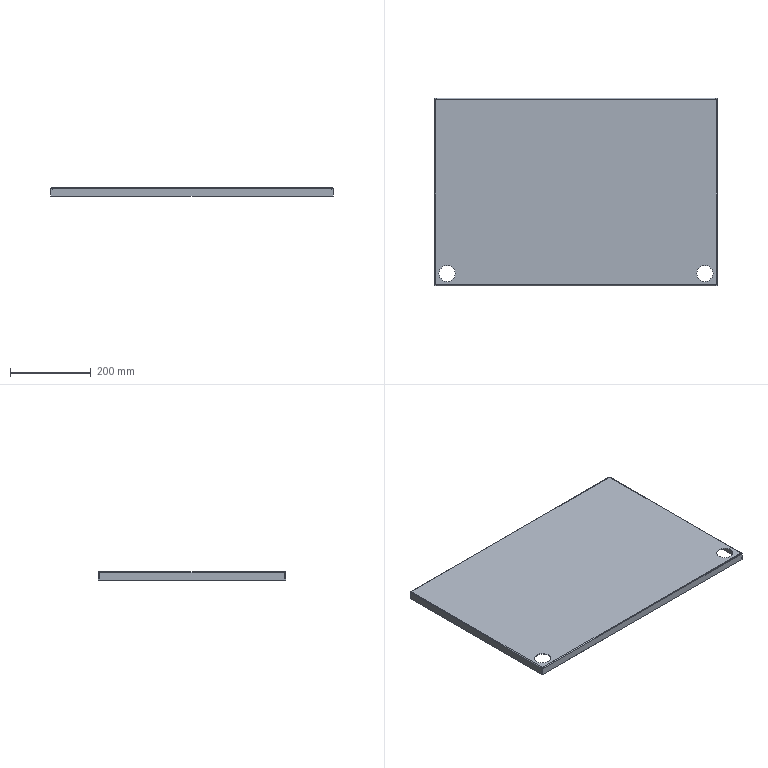Part | SolidWorks | features Extrusion 1, FlatPattern 1, FlattenBends 1, ICE 1, ProcessBends 1, Rip 1, SheetMetal 1, Shell 1 | 1 solid | 62 faces | box 697 x 463 x 20 mm | volume 721539 mm3 | plane 54 | cylinder 8 | commonest cylinder face diameters 4 x4 40 x4